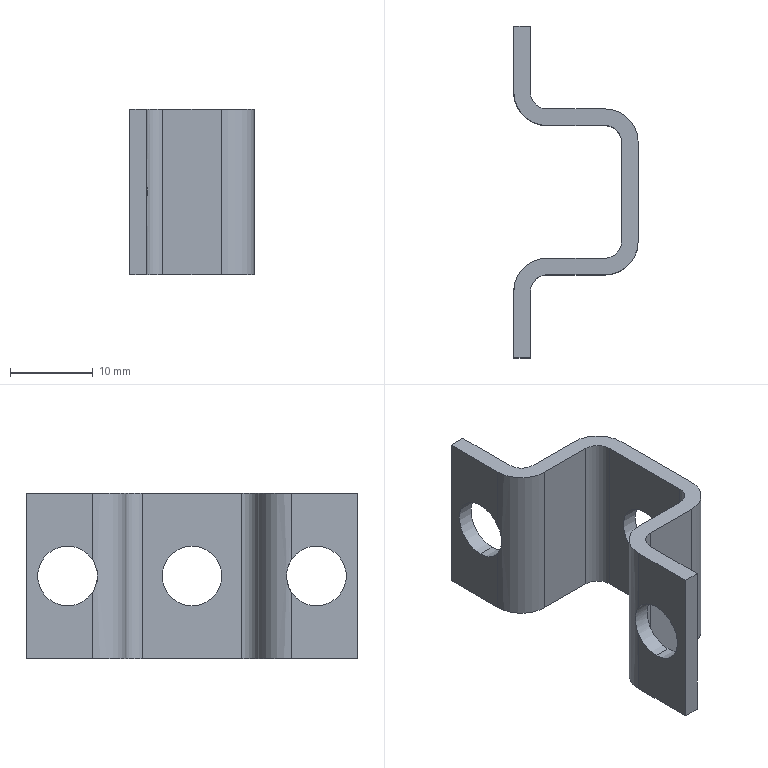Part | NX | features solid 2 | 1 solid | 28 faces | box 15 x 40 x 20 mm | volume 2190 mm3 | cylinder 14 | plane 14 | commonest cylinder face diameters 7.2 x6 4 x4 8 x4
STEP:
#1=CARTESIAN_POINT('',(-1106.,275.,348.4));
#2=VERTEX_POINT('',#1);
#3=CARTESIAN_POINT('',(-1108.,275.,348.4));
#4=VERTEX_POINT('',#3);
#5=CARTESIAN_POINT('',(-1140.17,275.,348.4));
#6=DIRECTION('',(1.,0.,0.));
#7=VECTOR('',#6,1000.);
#8=LINE('',#5,#7);
#9=EDGE_CURVE('',#2,#4,#8,.F.);
#10=ORIENTED_EDGE('',*,*,#9,.T.);
#11=CARTESIAN_POINT('',(-1108.,275.,355.6));
#12=VERTEX_POINT('',#11);
#13=CARTESIAN_POINT('',(-1108.,275.,352.));
#14=DIRECTION('',(-1.,0.,0.));
#15=DIRECTION('',(0.,-1.,0.));
#16=AXIS2_PLACEMENT_3D('',#13,#14,#15);
#17=CIRCLE('',#16,3.6);
#18=EDGE_CURVE('',#4,#12,#17,.T.);
#19=ORIENTED_EDGE('',*,*,#18,.T.);
#20=CARTESIAN_POINT('',(-1106.,275.,355.6));
#21=VERTEX_POINT('',#20);
#22=CARTESIAN_POINT('',(-1140.17,275.,355.6));
#23=DIRECTION('',(1.,0.,0.));
#24=VECTOR('',#23,1000.);
#25=LINE('',#22,#24);
#26=EDGE_CURVE('',#12,#21,#25,.T.);
#27=ORIENTED_EDGE('',*,*,#26,.T.);
#28=CARTESIAN_POINT('',(-1106.,275.,352.));
#29=DIRECTION('',(-1.,0.,0.));
#30=DIRECTION('',(0.,-1.,0.));
#31=AXIS2_PLACEMENT_3D('',#28,#29,#30);
#32=CIRCLE('',#31,3.6);
#33=EDGE_CURVE('',#2,#21,#32,.T.);
#34=ORIENTED_EDGE('',*,*,#33,.F.);
#35=EDGE_LOOP('',(#10,#19,#27,#34));
#36=FACE_BOUND('',#35,.T.);
#37=CARTESIAN_POINT('',(-1140.17,275.,352.));
#38=DIRECTION('',(1.,0.,0.));
#39=DIRECTION('',(0.,0.,1.));
#40=AXIS2_PLACEMENT_3D('',#37,#38,#39);
#41=CYLINDRICAL_SURFACE('',#40,3.6);
#42=ADVANCED_FACE('',(#36),#41,.F.);
#43=CARTESIAN_POINT('',(-1108.,305.,348.4));
#44=VERTEX_POINT('',#43);
#45=CARTESIAN_POINT('',(-1106.,305.,348.4));
#46=VERTEX_POINT('',#45);
#47=CARTESIAN_POINT('',(-1140.17,305.,348.4));
#48=DIRECTION('',(1.,0.,0.));
#49=VECTOR('',#48,1000.);
#50=LINE('',#47,#49);
#51=EDGE_CURVE('',#44,#46,#50,.T.);
#52=ORIENTED_EDGE('',*,*,#51,.F.);
#53=CARTESIAN_POINT('',(-1108.,302.,350.01));
#54=VERTEX_POINT('',#53);
#55=CARTESIAN_POINT('',(-1108.,305.,352.));
#56=DIRECTION('',(-1.,0.,0.));
#57=DIRECTION('',(0.,-1.,0.));
#58=AXIS2_PLACEMENT_3D('',#55,#56,#57);
#59=CIRCLE('',#58,3.6);
#60=EDGE_CURVE('',#44,#54,#59,.T.);
#61=ORIENTED_EDGE('',*,*,#60,.T.);
#62=CARTESIAN_POINT('',(-1108.,302.,353.99));
#63=VERTEX_POINT('',#62);
#64=CARTESIAN_POINT('',(-1108.,302.,350.01));
#65=CARTESIAN_POINT('',(-1108.,301.934,350.109));
#66=CARTESIAN_POINT('',(-1107.997,301.783,350.353));
#67=CARTESIAN_POINT('',(-1107.977,301.531,350.955));
#68=CARTESIAN_POINT('',(-1107.958,301.408,351.604));
#69=CARTESIAN_POINT('',(-1107.953,301.396,351.997));
#70=CARTESIAN_POINT('',(-1107.958,301.408,352.39));
#71=CARTESIAN_POINT('',(-1107.977,301.53,353.043));
#72=CARTESIAN_POINT('',(-1107.997,301.783,353.647));
#73=CARTESIAN_POINT('',(-1108.,301.935,353.891));
#74=CARTESIAN_POINT('',(-1108.,302.,353.99));
#75=B_SPLINE_CURVE_WITH_KNOTS('',3,(#64,#65,#66,#67,#68,#69,#70,#71,#72,#73,#74),.UNSPECIFIED.,.F.,.F.,(4,1,1,1,1,1,1,1,4),(0.,0.125,0.25,0.375,0.5,0.625,0.75,0.875,1.),.UNSPECIFIED.);
#76=EDGE_CURVE('',#54,#63,#75,.T.);
#77=ORIENTED_EDGE('',*,*,#76,.T.);
#78=CARTESIAN_POINT('',(-1108.,305.,355.6));
#79=VERTEX_POINT('',#78);
#80=CARTESIAN_POINT('',(-1108.,305.,352.));
#81=DIRECTION('',(-1.,0.,0.));
#82=DIRECTION('',(0.,-1.,0.));
#83=AXIS2_PLACEMENT_3D('',#80,#81,#82);
#84=CIRCLE('',#83,3.6);
#85=EDGE_CURVE('',#63,#79,#84,.T.);
#86=ORIENTED_EDGE('',*,*,#85,.T.);
#87=CARTESIAN_POINT('',(-1106.,305.,355.6));
#88=VERTEX_POINT('',#87);
#89=CARTESIAN_POINT('',(-1140.17,305.,355.6));
#90=DIRECTION('',(1.,0.,0.));
#91=VECTOR('',#90,1000.);
#92=LINE('',#89,#91);
#93=EDGE_CURVE('',#88,#79,#92,.F.);
#94=ORIENTED_EDGE('',*,*,#93,.F.);
#95=CARTESIAN_POINT('',(-1106.,302.,353.99));
#96=VERTEX_POINT('',#95);
#97=CARTESIAN_POINT('',(-1106.,305.,352.));
#98=DIRECTION('',(-1.,0.,0.));
#99=DIRECTION('',(0.,-1.,0.));
#100=AXIS2_PLACEMENT_3D('',#97,#98,#99);
#101=CIRCLE('',#100,3.6);
#102=EDGE_CURVE('',#96,#88,#101,.T.);
#103=ORIENTED_EDGE('',*,*,#102,.F.);
#104=CARTESIAN_POINT('',(-1106.,302.,350.01));
#105=VERTEX_POINT('',#104);
#106=CARTESIAN_POINT('',(-1106.,302.,353.99));
#107=CARTESIAN_POINT('',(-1106.,301.948,353.912));
#108=CARTESIAN_POINT('',(-1105.993,301.807,353.704));
#109=CARTESIAN_POINT('',(-1105.929,301.427,352.772));
#110=CARTESIAN_POINT('',(-1105.894,301.382,351.998));
#111=CARTESIAN_POINT('',(-1105.929,301.428,351.227));
#112=CARTESIAN_POINT('',(-1105.993,301.808,350.296));
#113=CARTESIAN_POINT('',(-1106.,301.948,350.088));
#114=CARTESIAN_POINT('',(-1106.,302.,350.01));
#115=B_SPLINE_CURVE_WITH_KNOTS('',3,(#106,#107,#108,#109,#110,#111,#112,#113,#114),.UNSPECIFIED.,.F.,.F.,(4,1,1,1,1,1,4),(0.,0.125,0.25,0.5,0.75,0.875,1.),.UNSPECIFIED.);
#116=EDGE_CURVE('',#105,#96,#115,.F.);
#117=ORIENTED_EDGE('',*,*,#116,.F.);
#118=CARTESIAN_POINT('',(-1106.,305.,352.));
#119=DIRECTION('',(-1.,0.,0.));
#120=DIRECTION('',(0.,-1.,0.));
#121=AXIS2_PLACEMENT_3D('',#118,#119,#120);
#122=CIRCLE('',#121,3.6);
#123=EDGE_CURVE('',#46,#105,#122,.T.);
#124=ORIENTED_EDGE('',*,*,#123,.F.);
#125=EDGE_LOOP('',(#52,#61,#77,#86,#94,#103,#117,#124));
#126=FACE_BOUND('',#125,.T.);
#127=CARTESIAN_POINT('',(-1140.17,305.,352.));
#128=DIRECTION('',(1.,0.,0.));
#129=DIRECTION('',(0.,0.,1.));
#130=AXIS2_PLACEMENT_3D('',#127,#128,#129);
#131=CYLINDRICAL_SURFACE('',#130,3.6);
#132=ADVANCED_FACE('',(#126),#131,.F.);
#133=CARTESIAN_POINT('',(-1095.,290.,348.4));
#134=VERTEX_POINT('',#133);
#135=CARTESIAN_POINT('',(-1093.,290.,348.4));
#136=VERTEX_POINT('',#135);
#137=CARTESIAN_POINT('',(-1140.17,290.,348.4));
#138=DIRECTION('',(1.,0.,0.));
#139=VECTOR('',#138,1000.);
#140=LINE('',#137,#139);
#141=EDGE_CURVE('',#134,#136,#140,.T.);
#142=ORIENTED_EDGE('',*,*,#141,.F.);
#143=CARTESIAN_POINT('',(-1095.,290.,355.6));
#144=VERTEX_POINT('',#143);
#145=CARTESIAN_POINT('',(-1095.,290.,352.));
#146=DIRECTION('',(-1.,0.,0.));
#147=DIRECTION('',(0.,0.,-1.));
#148=AXIS2_PLACEMENT_3D('',#145,#146,#147);
#149=CIRCLE('',#148,3.6);
#150=EDGE_CURVE('',#134,#144,#149,.T.);
#151=ORIENTED_EDGE('',*,*,#150,.T.);
#152=CARTESIAN_POINT('',(-1093.,290.,355.6));
#153=VERTEX_POINT('',#152);
#154=CARTESIAN_POINT('',(-1140.17,290.,355.6));
#155=DIRECTION('',(1.,0.,0.));
#156=VECTOR('',#155,1000.);
#157=LINE('',#154,#156);
#158=EDGE_CURVE('',#153,#144,#157,.F.);
#159=ORIENTED_EDGE('',*,*,#158,.F.);
#160=CARTESIAN_POINT('',(-1093.,290.,352.));
#161=DIRECTION('',(1.,0.,0.));
#162=DIRECTION('',(0.,-1.,0.));
#163=AXIS2_PLACEMENT_3D('',#160,#161,#162);
#164=CIRCLE('',#163,3.6);
#165=EDGE_CURVE('',#153,#136,#164,.T.);
#166=ORIENTED_EDGE('',*,*,#165,.T.);
#167=EDGE_LOOP('',(#142,#151,#159,#166));
#168=FACE_BOUND('',#167,.T.);
#169=CARTESIAN_POINT('',(-1140.17,290.,352.));
#170=DIRECTION('',(1.,0.,0.));
#171=DIRECTION('',(0.,0.,1.));
#172=AXIS2_PLACEMENT_3D('',#169,#170,#171);
#173=CYLINDRICAL_SURFACE('',#172,3.6);
#174=ADVANCED_FACE('',(#168),#173,.F.);
#175=CARTESIAN_POINT('',(-1106.,302.,342.));
#176=VERTEX_POINT('',#175);
#177=CARTESIAN_POINT('',(-1106.,302.,342.));
#178=DIRECTION('',(0.,0.,1.));
#179=VECTOR('',#178,1000.);
#180=LINE('',#177,#179);
#181=EDGE_CURVE('',#176,#105,#180,.T.);
#182=ORIENTED_EDGE('',*,*,#181,.T.);
#183=ORIENTED_EDGE('',*,*,#116,.T.);
#184=CARTESIAN_POINT('',(-1106.,302.,362.));
#185=VERTEX_POINT('',#184);
#186=CARTESIAN_POINT('',(-1106.,302.,342.));
#187=DIRECTION('',(0.,0.,1.));
#188=VECTOR('',#187,1000.);
#189=LINE('',#186,#188);
#190=EDGE_CURVE('',#96,#185,#189,.T.);
#191=ORIENTED_EDGE('',*,*,#190,.T.);
#192=CARTESIAN_POINT('',(-1104.,300.,362.));
#193=VERTEX_POINT('',#192);
#194=CARTESIAN_POINT('',(-1104.,302.,362.));
#195=DIRECTION('',(0.,0.,1.));
#196=DIRECTION('',(1.,0.,0.));
#197=AXIS2_PLACEMENT_3D('',#194,#195,#196);
#198=CIRCLE('',#197,2.);
#199=EDGE_CURVE('',#185,#193,#198,.T.);
#200=ORIENTED_EDGE('',*,*,#199,.T.);
#201=CARTESIAN_POINT('',(-1104.,300.,342.));
#202=VERTEX_POINT('',#201);
#203=CARTESIAN_POINT('',(-1104.,300.,362.));
#204=DIRECTION('',(0.,0.,-1.));
#205=VECTOR('',#204,1000.);
#206=LINE('',#203,#205);
#207=EDGE_CURVE('',#193,#202,#206,.T.);
#208=ORIENTED_EDGE('',*,*,#207,.T.);
#209=CARTESIAN_POINT('',(-1104.,302.,342.));
#210=DIRECTION('',(0.,0.,1.));
#211=DIRECTION('',(1.,0.,0.));
#212=AXIS2_PLACEMENT_3D('',#209,#210,#211);
#213=CIRCLE('',#212,2.);
#214=EDGE_CURVE('',#176,#202,#213,.T.);
#215=ORIENTED_EDGE('',*,*,#214,.F.);
#216=EDGE_LOOP('',(#182,#183,#191,#200,#208,#215));
#217=FACE_BOUND('',#216,.T.);
#218=CARTESIAN_POINT('',(-1104.,302.,362.));
#219=DIRECTION('',(0.,0.,-1.));
#220=DIRECTION('',(0.,1.,0.));
#221=AXIS2_PLACEMENT_3D('',#218,#219,#220);
#222=CYLINDRICAL_SURFACE('',#221,2.);
#223=ADVANCED_FACE('',(#217),#222,.F.);
#224=ORIENTED_EDGE('',*,*,#76,.F.);
#225=CARTESIAN_POINT('',(-1108.,302.,342.));
#226=VERTEX_POINT('',#225);
#227=CARTESIAN_POINT('',(-1108.,302.,342.));
#228=DIRECTION('',(0.,0.,1.));
#229=VECTOR('',#228,1000.);
#230=LINE('',#227,#229);
#231=EDGE_CURVE('',#226,#54,#230,.T.);
#232=ORIENTED_EDGE('',*,*,#231,.F.);
#233=CARTESIAN_POINT('',(-1104.,298.,342.));
#234=VERTEX_POINT('',#233);
#235=CARTESIAN_POINT('',(-1104.,302.,342.));
#236=DIRECTION('',(0.,0.,1.));
#237=DIRECTION('',(0.,1.,0.));
#238=AXIS2_PLACEMENT_3D('',#235,#236,#237);
#239=CIRCLE('',#238,4.);
#240=EDGE_CURVE('',#226,#234,#239,.T.);
#241=ORIENTED_EDGE('',*,*,#240,.T.);
#242=CARTESIAN_POINT('',(-1104.,298.,362.));
#243=VERTEX_POINT('',#242);
#244=CARTESIAN_POINT('',(-1104.,298.,362.));
#245=DIRECTION('',(0.,0.,-1.));
#246=VECTOR('',#245,1000.);
#247=LINE('',#244,#246);
#248=EDGE_CURVE('',#243,#234,#247,.T.);
#249=ORIENTED_EDGE('',*,*,#248,.F.);
#250=CARTESIAN_POINT('',(-1108.,302.,362.));
#251=VERTEX_POINT('',#250);
#252=CARTESIAN_POINT('',(-1104.,302.,362.));
#253=DIRECTION('',(0.,0.,1.));
#254=DIRECTION('',(0.,1.,0.));
#255=AXIS2_PLACEMENT_3D('',#252,#253,#254);
#256=CIRCLE('',#255,4.);
#257=EDGE_CURVE('',#251,#243,#256,.T.);
#258=ORIENTED_EDGE('',*,*,#257,.F.);
#259=CARTESIAN_POINT('',(-1108.,302.,342.));
#260=DIRECTION('',(0.,0.,1.));
#261=VECTOR('',#260,1000.);
#262=LINE('',#259,#261);
#263=EDGE_CURVE('',#63,#251,#262,.T.);
#264=ORIENTED_EDGE('',*,*,#263,.F.);
#265=EDGE_LOOP('',(#224,#232,#241,#249,#258,#264));
#266=FACE_BOUND('',#265,.T.);
#267=CARTESIAN_POINT('',(-1104.,302.,362.));
#268=DIRECTION('',(0.,0.,-1.));
#269=DIRECTION('',(0.,1.,0.));
#270=AXIS2_PLACEMENT_3D('',#267,#268,#269);
#271=CYLINDRICAL_SURFACE('',#270,4.);
#272=ADVANCED_FACE('',(#266),#271,.T.);
#273=CARTESIAN_POINT('',(-1106.,310.,362.));
#274=VERTEX_POINT('',#273);
#275=CARTESIAN_POINT('',(-1106.,310.,342.));
#276=VERTEX_POINT('',#275);
#277=CARTESIAN_POINT('',(-1106.,310.,362.));
#278=DIRECTION('',(0.,0.,-1.));
#279=VECTOR('',#278,1000.);
#280=LINE('',#277,#279);
#281=EDGE_CURVE('',#274,#276,#280,.T.);
#282=ORIENTED_EDGE('',*,*,#281,.T.);
#283=CARTESIAN_POINT('',(-1108.,310.,342.));
#284=VERTEX_POINT('',#283);
#285=CARTESIAN_POINT('',(-1108.,310.,342.));
#286=DIRECTION('',(1.,0.,0.));
#287=VECTOR('',#286,1000.);
#288=LINE('',#285,#287);
#289=EDGE_CURVE('',#284,#276,#288,.T.);
#290=ORIENTED_EDGE('',*,*,#289,.F.);
#291=CARTESIAN_POINT('',(-1108.,310.,362.));
#292=VERTEX_POINT('',#291);
#293=CARTESIAN_POINT('',(-1108.,310.,362.));
#294=DIRECTION('',(0.,0.,-1.));
#295=VECTOR('',#294,1000.);
#296=LINE('',#293,#295);
#297=EDGE_CURVE('',#292,#284,#296,.T.);
#298=ORIENTED_EDGE('',*,*,#297,.F.);
#299=CARTESIAN_POINT('',(-1108.,310.,362.));
#300=DIRECTION('',(1.,0.,0.));
#301=VECTOR('',#300,1000.);
#302=LINE('',#299,#301);
#303=EDGE_CURVE('',#292,#274,#302,.T.);
#304=ORIENTED_EDGE('',*,*,#303,.T.);
#305=EDGE_LOOP('',(#282,#290,#298,#304));
#306=FACE_BOUND('',#305,.T.);
#307=CARTESIAN_POINT('',(-1108.,310.,362.));
#308=DIRECTION('',(0.,-1.,0.));
#309=DIRECTION('',(0.,0.,-1.));
#310=AXIS2_PLACEMENT_3D('',#307,#308,#309);
#311=PLANE('',#310);
#312=ADVANCED_FACE('',(#306),#311,.F.);
#313=ORIENTED_EDGE('',*,*,#190,.F.);
#314=ORIENTED_EDGE('',*,*,#102,.T.);
#315=CARTESIAN_POINT('',(-1106.,305.,352.));
#316=DIRECTION('',(-1.,0.,0.));
#317=DIRECTION('',(0.,-1.,0.));
#318=AXIS2_PLACEMENT_3D('',#315,#316,#317);
#319=CIRCLE('',#318,3.6);
#320=EDGE_CURVE('',#88,#46,#319,.T.);
#321=ORIENTED_EDGE('',*,*,#320,.T.);
#322=ORIENTED_EDGE('',*,*,#123,.T.);
#323=ORIENTED_EDGE('',*,*,#181,.F.);
#324=CARTESIAN_POINT('',(-1106.,299.722,342.));
#325=DIRECTION('',(0.,-1.,0.));
#326=VECTOR('',#325,1000.);
#327=LINE('',#324,#326);
#328=EDGE_CURVE('',#276,#176,#327,.T.);
#329=ORIENTED_EDGE('',*,*,#328,.F.);
#330=ORIENTED_EDGE('',*,*,#281,.F.);
#331=CARTESIAN_POINT('',(-1106.,299.722,362.));
#332=DIRECTION('',(0.,1.,0.));
#333=VECTOR('',#332,1000.);
#334=LINE('',#331,#333);
#335=EDGE_CURVE('',#185,#274,#334,.T.);
#336=ORIENTED_EDGE('',*,*,#335,.F.);
#337=EDGE_LOOP('',(#313,#314,#321,#322,#323,#329,#330,#336));
#338=FACE_BOUND('',#337,.T.);
#339=CARTESIAN_POINT('',(-1106.,290.,352.));
#340=DIRECTION('',(-1.,0.,0.));
#341=DIRECTION('',(0.,1.,0.));
#342=AXIS2_PLACEMENT_3D('',#339,#340,#341);
#343=PLANE('',#342);
#344=ADVANCED_FACE('',(#338),#343,.F.);
#345=ORIENTED_EDGE('',*,*,#85,.F.);
#346=ORIENTED_EDGE('',*,*,#263,.T.);
#347=CARTESIAN_POINT('',(-1108.,299.722,362.));
#348=DIRECTION('',(0.,1.,0.));
#349=VECTOR('',#348,1000.);
#350=LINE('',#347,#349);
#351=EDGE_CURVE('',#251,#292,#350,.T.);
#352=ORIENTED_EDGE('',*,*,#351,.T.);
#353=ORIENTED_EDGE('',*,*,#297,.T.);
#354=CARTESIAN_POINT('',(-1108.,299.722,342.));
#355=DIRECTION('',(0.,-1.,0.));
#356=VECTOR('',#355,1000.);
#357=LINE('',#354,#356);
#358=EDGE_CURVE('',#284,#226,#357,.T.);
#359=ORIENTED_EDGE('',*,*,#358,.T.);
#360=ORIENTED_EDGE('',*,*,#231,.T.);
#361=ORIENTED_EDGE('',*,*,#60,.F.);
#362=CARTESIAN_POINT('',(-1108.,305.,352.));
#363=DIRECTION('',(-1.,0.,0.));
#364=DIRECTION('',(0.,-1.,0.));
#365=AXIS2_PLACEMENT_3D('',#362,#363,#364);
#366=CIRCLE('',#365,3.6);
#367=EDGE_CURVE('',#79,#44,#366,.T.);
#368=ORIENTED_EDGE('',*,*,#367,.F.);
#369=EDGE_LOOP('',(#345,#346,#352,#353,#359,#360,#361,#368));
#370=FACE_BOUND('',#369,.T.);
#371=CARTESIAN_POINT('',(-1108.,290.,352.));
#372=DIRECTION('',(-1.,0.,0.));
#373=DIRECTION('',(0.,1.,0.));
#374=AXIS2_PLACEMENT_3D('',#371,#372,#373);
#375=PLANE('',#374);
#376=ADVANCED_FACE('',(#370),#375,.T.);
#377=CARTESIAN_POINT('',(-1106.,278.,362.));
#378=VERTEX_POINT('',#377);
#379=CARTESIAN_POINT('',(-1106.,278.,353.99));
#380=VERTEX_POINT('',#379);
#381=CARTESIAN_POINT('',(-1106.,278.,362.));
#382=DIRECTION('',(0.,0.,-1.));
#383=VECTOR('',#382,1000.);
#384=LINE('',#381,#383);
#385=EDGE_CURVE('',#378,#380,#384,.T.);
#386=ORIENTED_EDGE('',*,*,#385,.T.);
#387=CARTESIAN_POINT('',(-1106.,278.,350.01));
#388=VERTEX_POINT('',#387);
#389=CARTESIAN_POINT('',(-1106.,278.,353.99));
#390=CARTESIAN_POINT('',(-1106.,278.406,353.378));
#391=CARTESIAN_POINT('',(-1105.816,278.794,352.002));
#392=CARTESIAN_POINT('',(-1106.,278.406,350.623));
#393=CARTESIAN_POINT('',(-1106.,278.,350.01));
#394=B_SPLINE_CURVE_WITH_KNOTS('',3,(#389,#390,#391,#392,#393),.UNSPECIFIED.,.F.,.F.,(4,1,4),(0.,0.5,1.),.UNSPECIFIED.);
#395=EDGE_CURVE('',#380,#388,#394,.T.);
#396=ORIENTED_EDGE('',*,*,#395,.T.);
#397=CARTESIAN_POINT('',(-1106.,278.,342.));
#398=VERTEX_POINT('',#397);
#399=CARTESIAN_POINT('',(-1106.,278.,362.));
#400=DIRECTION('',(0.,0.,-1.));
#401=VECTOR('',#400,1000.);
#402=LINE('',#399,#401);
#403=EDGE_CURVE('',#388,#398,#402,.T.);
#404=ORIENTED_EDGE('',*,*,#403,.T.);
#405=CARTESIAN_POINT('',(-1104.,280.,342.));
#406=VERTEX_POINT('',#405);
#407=CARTESIAN_POINT('',(-1104.,278.,342.));
#408=DIRECTION('',(0.,0.,1.));
#409=DIRECTION('',(-1.,0.,0.));
#410=AXIS2_PLACEMENT_3D('',#407,#408,#409);
#411=CIRCLE('',#410,2.);
#412=EDGE_CURVE('',#406,#398,#411,.T.);
#413=ORIENTED_EDGE('',*,*,#412,.F.);
#414=CARTESIAN_POINT('',(-1104.,280.,362.));
#415=VERTEX_POINT('',#414);
#416=CARTESIAN_POINT('',(-1104.,280.,342.));
#417=DIRECTION('',(0.,0.,1.));
#418=VECTOR('',#417,1000.);
#419=LINE('',#416,#418);
#420=EDGE_CURVE('',#406,#415,#419,.T.);
#421=ORIENTED_EDGE('',*,*,#420,.T.);
#422=CARTESIAN_POINT('',(-1104.,278.,362.));
#423=DIRECTION('',(0.,0.,1.));
#424=DIRECTION('',(-1.,0.,0.));
#425=AXIS2_PLACEMENT_3D('',#422,#423,#424);
#426=CIRCLE('',#425,2.);
#427=EDGE_CURVE('',#415,#378,#426,.T.);
#428=ORIENTED_EDGE('',*,*,#427,.T.);
#429=EDGE_LOOP('',(#386,#396,#404,#413,#421,#428));
#430=FACE_BOUND('',#429,.T.);
#431=CARTESIAN_POINT('',(-1104.,278.,342.));
#432=DIRECTION('',(0.,0.,1.));
#433=DIRECTION('',(0.,-1.,0.));
#434=AXIS2_PLACEMENT_3D('',#431,#432,#433);
#435=CYLINDRICAL_SURFACE('',#434,2.);
#436=ADVANCED_FACE('',(#430),#435,.F.);
#437=CARTESIAN_POINT('',(-1108.,278.,353.99));
#438=VERTEX_POINT('',#437);
#439=CARTESIAN_POINT('',(-1108.,278.,350.01));
#440=VERTEX_POINT('',#439);
#441=CARTESIAN_POINT('',(-1108.,278.,350.01));
#442=CARTESIAN_POINT('',(-1108.,278.402,350.616));
#443=CARTESIAN_POINT('',(-1107.909,278.798,352.006));
#444=CARTESIAN_POINT('',(-1108.,278.401,353.385));
#445=CARTESIAN_POINT('',(-1108.,278.,353.99));
#446=B_SPLINE_CURVE_WITH_KNOTS('',3,(#441,#442,#443,#444,#445),.UNSPECIFIED.,.F.,.F.,(4,1,4),(0.,0.5,1.),.UNSPECIFIED.);
#447=EDGE_CURVE('',#438,#440,#446,.F.);
#448=ORIENTED_EDGE('',*,*,#447,.F.);
#449=CARTESIAN_POINT('',(-1108.,278.,362.));
#450=VERTEX_POINT('',#449);
#451=CARTESIAN_POINT('',(-1108.,278.,362.));
#452=DIRECTION('',(0.,0.,-1.));
#453=VECTOR('',#452,1000.);
#454=LINE('',#451,#453);
#455=EDGE_CURVE('',#450,#438,#454,.T.);
#456=ORIENTED_EDGE('',*,*,#455,.F.);
#457=CARTESIAN_POINT('',(-1104.,282.,362.));
#458=VERTEX_POINT('',#457);
#459=CARTESIAN_POINT('',(-1104.,278.,362.));
#460=DIRECTION('',(0.,0.,1.));
#461=DIRECTION('',(0.,-1.,0.));
#462=AXIS2_PLACEMENT_3D('',#459,#460,#461);
#463=CIRCLE('',#462,4.);
#464=EDGE_CURVE('',#458,#450,#463,.T.);
#465=ORIENTED_EDGE('',*,*,#464,.F.);
#466=CARTESIAN_POINT('',(-1104.,282.,342.));
#467=VERTEX_POINT('',#466);
#468=CARTESIAN_POINT('',(-1104.,282.,342.));
#469=DIRECTION('',(0.,0.,1.));
#470=VECTOR('',#469,1000.);
#471=LINE('',#468,#470);
#472=EDGE_CURVE('',#467,#458,#471,.T.);
#473=ORIENTED_EDGE('',*,*,#472,.F.);
#474=CARTESIAN_POINT('',(-1108.,278.,342.));
#475=VERTEX_POINT('',#474);
#476=CARTESIAN_POINT('',(-1104.,278.,342.));
#477=DIRECTION('',(0.,0.,1.));
#478=DIRECTION('',(0.,-1.,0.));
#479=AXIS2_PLACEMENT_3D('',#476,#477,#478);
#480=CIRCLE('',#479,4.);
#481=EDGE_CURVE('',#467,#475,#480,.T.);
#482=ORIENTED_EDGE('',*,*,#481,.T.);
#483=CARTESIAN_POINT('',(-1108.,278.,362.));
#484=DIRECTION('',(0.,0.,-1.));
#485=VECTOR('',#484,1000.);
#486=LINE('',#483,#485);
#487=EDGE_CURVE('',#440,#475,#486,.T.);
#488=ORIENTED_EDGE('',*,*,#487,.F.);
#489=EDGE_LOOP('',(#448,#456,#465,#473,#482,#488));
#490=FACE_BOUND('',#489,.T.);
#491=CARTESIAN_POINT('',(-1104.,278.,342.));
#492=DIRECTION('',(0.,0.,1.));
#493=DIRECTION('',(0.,-1.,0.));
#494=AXIS2_PLACEMENT_3D('',#491,#492,#493);
#495=CYLINDRICAL_SURFACE('',#494,4.);
#496=ADVANCED_FACE('',(#490),#495,.T.);
#497=CARTESIAN_POINT('',(-1106.,270.,342.));
#498=VERTEX_POINT('',#497);
#499=CARTESIAN_POINT('',(-1106.,270.,362.));
#500=VERTEX_POINT('',#499);
#501=CARTESIAN_POINT('',(-1106.,270.,342.));
#502=DIRECTION('',(0.,0.,1.));
#503=VECTOR('',#502,1000.);
#504=LINE('',#501,#503);
#505=EDGE_CURVE('',#498,#500,#504,.T.);
#506=ORIENTED_EDGE('',*,*,#505,.T.);
#507=CARTESIAN_POINT('',(-1108.,270.,362.));
#508=VERTEX_POINT('',#507);
#509=CARTESIAN_POINT('',(-1108.,270.,362.));
#510=DIRECTION('',(1.,0.,0.));
#511=VECTOR('',#510,1000.);
#512=LINE('',#509,#511);
#513=EDGE_CURVE('',#508,#500,#512,.T.);
#514=ORIENTED_EDGE('',*,*,#513,.F.);
#515=CARTESIAN_POINT('',(-1108.,270.,342.));
#516=VERTEX_POINT('',#515);
#517=CARTESIAN_POINT('',(-1108.,270.,342.));
#518=DIRECTION('',(0.,0.,1.));
#519=VECTOR('',#518,1000.);
#520=LINE('',#517,#519);
#521=EDGE_CURVE('',#516,#508,#520,.T.);
#522=ORIENTED_EDGE('',*,*,#521,.F.);
#523=CARTESIAN_POINT('',(-1108.,270.,342.));
#524=DIRECTION('',(1.,0.,0.));
#525=VECTOR('',#524,1000.);
#526=LINE('',#523,#525);
#527=EDGE_CURVE('',#516,#498,#526,.T.);
#528=ORIENTED_EDGE('',*,*,#527,.T.);
#529=EDGE_LOOP('',(#506,#514,#522,#528));
#530=FACE_BOUND('',#529,.T.);
#531=CARTESIAN_POINT('',(-1108.,270.,342.));
#532=DIRECTION('',(0.,1.,0.));
#533=DIRECTION('',(1.,0.,0.));
#534=AXIS2_PLACEMENT_3D('',#531,#532,#533);
#535=PLANE('',#534);
#536=ADVANCED_FACE('',(#530),#535,.F.);
#537=ORIENTED_EDGE('',*,*,#403,.F.);
#538=CARTESIAN_POINT('',(-1106.,275.,352.));
#539=DIRECTION('',(-1.,0.,0.));
#540=DIRECTION('',(0.,-1.,0.));
#541=AXIS2_PLACEMENT_3D('',#538,#539,#540);
#542=CIRCLE('',#541,3.6);
#543=EDGE_CURVE('',#388,#2,#542,.T.);
#544=ORIENTED_EDGE('',*,*,#543,.T.);
#545=ORIENTED_EDGE('',*,*,#33,.T.);
#546=CARTESIAN_POINT('',(-1106.,275.,352.));
#547=DIRECTION('',(-1.,0.,0.));
#548=DIRECTION('',(0.,-1.,0.));
#549=AXIS2_PLACEMENT_3D('',#546,#547,#548);
#550=CIRCLE('',#549,3.6);
#551=EDGE_CURVE('',#21,#380,#550,.T.);
#552=ORIENTED_EDGE('',*,*,#551,.T.);
#553=ORIENTED_EDGE('',*,*,#385,.F.);
#554=CARTESIAN_POINT('',(-1106.,280.278,362.));
#555=DIRECTION('',(0.,1.,0.));
#556=VECTOR('',#555,1000.);
#557=LINE('',#554,#556);
#558=EDGE_CURVE('',#500,#378,#557,.T.);
#559=ORIENTED_EDGE('',*,*,#558,.F.);
#560=ORIENTED_EDGE('',*,*,#505,.F.);
#561=CARTESIAN_POINT('',(-1106.,280.278,342.));
#562=DIRECTION('',(0.,-1.,0.));
#563=VECTOR('',#562,1000.);
#564=LINE('',#561,#563);
#565=EDGE_CURVE('',#398,#498,#564,.T.);
#566=ORIENTED_EDGE('',*,*,#565,.F.);
#567=EDGE_LOOP('',(#537,#544,#545,#552,#553,#559,#560,#566));
#568=FACE_BOUND('',#567,.T.);
#569=CARTESIAN_POINT('',(-1106.,290.,352.));
#570=DIRECTION('',(-1.,0.,0.));
#571=DIRECTION('',(0.,0.,1.));
#572=AXIS2_PLACEMENT_3D('',#569,#570,#571);
#573=PLANE('',#572);
#574=ADVANCED_FACE('',(#568),#573,.F.);
#575=CARTESIAN_POINT('',(-1108.,275.,352.));
#576=DIRECTION('',(-1.,0.,0.));
#577=DIRECTION('',(0.,-1.,0.));
#578=AXIS2_PLACEMENT_3D('',#575,#576,#577);
#579=CIRCLE('',#578,3.6);
#580=EDGE_CURVE('',#440,#4,#579,.T.);
#581=ORIENTED_EDGE('',*,*,#580,.F.);
#582=ORIENTED_EDGE('',*,*,#487,.T.);
#583=CARTESIAN_POINT('',(-1108.,280.278,342.));
#584=DIRECTION('',(0.,-1.,0.));
#585=VECTOR('',#584,1000.);
#586=LINE('',#583,#585);
#587=EDGE_CURVE('',#475,#516,#586,.T.);
#588=ORIENTED_EDGE('',*,*,#587,.T.);
#589=ORIENTED_EDGE('',*,*,#521,.T.);
#590=CARTESIAN_POINT('',(-1108.,280.278,362.));
#591=DIRECTION('',(0.,1.,0.));
#592=VECTOR('',#591,1000.);
#593=LINE('',#590,#592);
#594=EDGE_CURVE('',#508,#450,#593,.T.);
#595=ORIENTED_EDGE('',*,*,#594,.T.);
#596=ORIENTED_EDGE('',*,*,#455,.T.);
#597=CARTESIAN_POINT('',(-1108.,275.,352.));
#598=DIRECTION('',(-1.,0.,0.));
#599=DIRECTION('',(0.,-1.,0.));
#600=AXIS2_PLACEMENT_3D('',#597,#598,#599);
#601=CIRCLE('',#600,3.6);
#602=EDGE_CURVE('',#12,#438,#601,.T.);
#603=ORIENTED_EDGE('',*,*,#602,.F.);
#604=ORIENTED_EDGE('',*,*,#18,.F.);
#605=EDGE_LOOP('',(#581,#582,#588,#589,#595,#596,#603,#604));
#606=FACE_BOUND('',#605,.T.);
#607=CARTESIAN_POINT('',(-1108.,290.,352.));
#608=DIRECTION('',(-1.,0.,0.));
#609=DIRECTION('',(0.,0.,1.));
#610=AXIS2_PLACEMENT_3D('',#607,#608,#609);
#611=PLANE('',#610);
#612=ADVANCED_FACE('',(#606),#611,.T.);
#613=ORIENTED_EDGE('',*,*,#420,.F.);
#614=CARTESIAN_POINT('',(-1097.,280.,342.));
#615=VERTEX_POINT('',#614);
#616=CARTESIAN_POINT('',(-1108.,280.,342.));
#617=DIRECTION('',(-1.,0.,0.));
#618=VECTOR('',#617,1000.);
#619=LINE('',#616,#618);
#620=EDGE_CURVE('',#615,#406,#619,.T.);
#621=ORIENTED_EDGE('',*,*,#620,.F.);
#622=CARTESIAN_POINT('',(-1097.,280.,362.));
#623=VERTEX_POINT('',#622);
#624=CARTESIAN_POINT('',(-1097.,280.,342.));
#625=DIRECTION('',(0.,0.,1.));
#626=VECTOR('',#625,1000.);
#627=LINE('',#624,#626);
#628=EDGE_CURVE('',#615,#623,#627,.T.);
#629=ORIENTED_EDGE('',*,*,#628,.T.);
#630=CARTESIAN_POINT('',(-1108.,280.,362.));
#631=DIRECTION('',(-1.,0.,0.));
#632=VECTOR('',#631,1000.);
#633=LINE('',#630,#632);
#634=EDGE_CURVE('',#623,#415,#633,.T.);
#635=ORIENTED_EDGE('',*,*,#634,.T.);
#636=EDGE_LOOP('',(#613,#621,#629,#635));
#637=FACE_BOUND('',#636,.T.);
#638=CARTESIAN_POINT('',(-1108.,280.,342.));
#639=DIRECTION('',(0.,1.,0.));
#640=DIRECTION('',(1.,0.,0.));
#641=AXIS2_PLACEMENT_3D('',#638,#639,#640);
#642=PLANE('',#641);
#643=ADVANCED_FACE('',(#637),#642,.F.);
#644=CARTESIAN_POINT('',(-1093.,284.,362.));
#645=VERTEX_POINT('',#644);
#646=CARTESIAN_POINT('',(-1097.,284.,362.));
#647=DIRECTION('',(0.,0.,-1.));
#648=DIRECTION('',(-1.,0.,0.));
#649=AXIS2_PLACEMENT_3D('',#646,#647,#648);
#650=CIRCLE('',#649,4.);
#651=EDGE_CURVE('',#645,#623,#650,.T.);
#652=ORIENTED_EDGE('',*,*,#651,.T.);
#653=ORIENTED_EDGE('',*,*,#628,.F.);
#654=CARTESIAN_POINT('',(-1093.,284.,342.));
#655=VERTEX_POINT('',#654);
#656=CARTESIAN_POINT('',(-1097.,284.,342.));
#657=DIRECTION('',(0.,0.,-1.));
#658=DIRECTION('',(-1.,0.,0.));
#659=AXIS2_PLACEMENT_3D('',#656,#657,#658);
#660=CIRCLE('',#659,4.);
#661=EDGE_CURVE('',#655,#615,#660,.T.);
#662=ORIENTED_EDGE('',*,*,#661,.F.);
#663=CARTESIAN_POINT('',(-1093.,284.,342.));
#664=DIRECTION('',(0.,0.,1.));
#665=VECTOR('',#664,1000.);
#666=LINE('',#663,#665);
#667=EDGE_CURVE('',#655,#645,#666,.T.);
#668=ORIENTED_EDGE('',*,*,#667,.T.);
#669=EDGE_LOOP('',(#652,#653,#662,#668));
#670=FACE_BOUND('',#669,.T.);
#671=CARTESIAN_POINT('',(-1097.,284.,342.));
#672=DIRECTION('',(0.,0.,1.));
#673=DIRECTION('',(-1.,0.,0.));
#674=AXIS2_PLACEMENT_3D('',#671,#672,#673);
#675=CYLINDRICAL_SURFACE('',#674,4.);
#676=ADVANCED_FACE('',(#670),#675,.T.);
#677=ORIENTED_EDGE('',*,*,#165,.F.);
#678=CARTESIAN_POINT('',(-1093.,290.,352.));
#679=DIRECTION('',(1.,0.,0.));
#680=DIRECTION('',(0.,-1.,0.));
#681=AXIS2_PLACEMENT_3D('',#678,#679,#680);
#682=CIRCLE('',#681,3.6);
#683=EDGE_CURVE('',#136,#153,#682,.T.);
#684=ORIENTED_EDGE('',*,*,#683,.F.);
#685=EDGE_LOOP('',(#677,#684));
#686=FACE_BOUND('',#685,.T.);
#687=CARTESIAN_POINT('',(-1093.,296.,362.));
#688=VERTEX_POINT('',#687);
#689=CARTESIAN_POINT('',(-1093.,280.,362.));
#690=DIRECTION('',(0.,-1.,0.));
#691=VECTOR('',#690,1000.);
#692=LINE('',#689,#691);
#693=EDGE_CURVE('',#688,#645,#692,.T.);
#694=ORIENTED_EDGE('',*,*,#693,.T.);
#695=ORIENTED_EDGE('',*,*,#667,.F.);
#696=CARTESIAN_POINT('',(-1093.,296.,342.));
#697=VERTEX_POINT('',#696);
#698=CARTESIAN_POINT('',(-1093.,280.,342.));
#699=DIRECTION('',(0.,-1.,0.));
#700=VECTOR('',#699,1000.);
#701=LINE('',#698,#700);
#702=EDGE_CURVE('',#697,#655,#701,.T.);
#703=ORIENTED_EDGE('',*,*,#702,.F.);
#704=CARTESIAN_POINT('',(-1093.,296.,342.));
#705=DIRECTION('',(0.,0.,1.));
#706=VECTOR('',#705,1000.);
#707=LINE('',#704,#706);
#708=EDGE_CURVE('',#697,#688,#707,.T.);
#709=ORIENTED_EDGE('',*,*,#708,.T.);
#710=EDGE_LOOP('',(#694,#695,#703,#709));
#711=FACE_BOUND('',#710,.T.);
#712=CARTESIAN_POINT('',(-1093.,280.,342.));
#713=DIRECTION('',(-1.,0.,0.));
#714=DIRECTION('',(0.,0.,1.));
#715=AXIS2_PLACEMENT_3D('',#712,#713,#714);
#716=PLANE('',#715);
#717=ADVANCED_FACE('',(#686,#711),#716,.F.);
#718=CARTESIAN_POINT('',(-1097.,300.,362.));
#719=VERTEX_POINT('',#718);
#720=CARTESIAN_POINT('',(-1097.,296.,362.));
#721=DIRECTION('',(0.,0.,-1.));
#722=DIRECTION('',(-1.,0.,0.));
#723=AXIS2_PLACEMENT_3D('',#720,#721,#722);
#724=CIRCLE('',#723,4.);
#725=EDGE_CURVE('',#719,#688,#724,.T.);
#726=ORIENTED_EDGE('',*,*,#725,.T.);
#727=ORIENTED_EDGE('',*,*,#708,.F.);
#728=CARTESIAN_POINT('',(-1097.,300.,342.));
#729=VERTEX_POINT('',#728);
#730=CARTESIAN_POINT('',(-1097.,296.,342.));
#731=DIRECTION('',(0.,0.,-1.));
#732=DIRECTION('',(-1.,0.,0.));
#733=AXIS2_PLACEMENT_3D('',#730,#731,#732);
#734=CIRCLE('',#733,4.);
#735=EDGE_CURVE('',#729,#697,#734,.T.);
#736=ORIENTED_EDGE('',*,*,#735,.F.);
#737=CARTESIAN_POINT('',(-1097.,300.,342.));
#738=DIRECTION('',(0.,0.,1.));
#739=VECTOR('',#738,1000.);
#740=LINE('',#737,#739);
#741=EDGE_CURVE('',#729,#719,#740,.T.);
#742=ORIENTED_EDGE('',*,*,#741,.T.);
#743=EDGE_LOOP('',(#726,#727,#736,#742));
#744=FACE_BOUND('',#743,.T.);
#745=CARTESIAN_POINT('',(-1097.,296.,342.));
#746=DIRECTION('',(0.,0.,1.));
#747=DIRECTION('',(-1.,0.,0.));
#748=AXIS2_PLACEMENT_3D('',#745,#746,#747);
#749=CYLINDRICAL_SURFACE('',#748,4.);
#750=ADVANCED_FACE('',(#744),#749,.T.);
#751=ORIENTED_EDGE('',*,*,#207,.F.);
#752=CARTESIAN_POINT('',(-1093.,300.,362.));
#753=DIRECTION('',(1.,0.,0.));
#754=VECTOR('',#753,1000.);
#755=LINE('',#752,#754);
#756=EDGE_CURVE('',#193,#719,#755,.T.);
#757=ORIENTED_EDGE('',*,*,#756,.T.);
#758=ORIENTED_EDGE('',*,*,#741,.F.);
#759=CARTESIAN_POINT('',(-1093.,300.,342.));
#760=DIRECTION('',(1.,0.,0.));
#761=VECTOR('',#760,1000.);
#762=LINE('',#759,#761);
#763=EDGE_CURVE('',#202,#729,#762,.T.);
#764=ORIENTED_EDGE('',*,*,#763,.F.);
#765=EDGE_LOOP('',(#751,#757,#758,#764));
#766=FACE_BOUND('',#765,.T.);
#767=CARTESIAN_POINT('',(-1093.,300.,342.));
#768=DIRECTION('',(0.,-1.,0.));
#769=DIRECTION('',(0.,0.,-1.));
#770=AXIS2_PLACEMENT_3D('',#767,#768,#769);
#771=PLANE('',#770);
#772=ADVANCED_FACE('',(#766),#771,.F.);
#773=CARTESIAN_POINT('',(-1095.,284.,362.));
#774=VERTEX_POINT('',#773);
#775=CARTESIAN_POINT('',(-1097.,282.,362.));
#776=VERTEX_POINT('',#775);
#777=CARTESIAN_POINT('',(-1097.,284.,362.));
#778=DIRECTION('',(0.,0.,-1.));
#779=DIRECTION('',(-1.,0.,0.));
#780=AXIS2_PLACEMENT_3D('',#777,#778,#779);
#781=CIRCLE('',#780,2.);
#782=EDGE_CURVE('',#774,#776,#781,.T.);
#783=ORIENTED_EDGE('',*,*,#782,.F.);
#784=CARTESIAN_POINT('',(-1095.,284.,342.));
#785=VERTEX_POINT('',#784);
#786=CARTESIAN_POINT('',(-1095.,284.,342.));
#787=DIRECTION('',(0.,0.,1.));
#788=VECTOR('',#787,1000.);
#789=LINE('',#786,#788);
#790=EDGE_CURVE('',#785,#774,#789,.T.);
#791=ORIENTED_EDGE('',*,*,#790,.F.);
#792=CARTESIAN_POINT('',(-1097.,282.,342.));
#793=VERTEX_POINT('',#792);
#794=CARTESIAN_POINT('',(-1097.,284.,342.));
#795=DIRECTION('',(0.,0.,-1.));
#796=DIRECTION('',(-1.,0.,0.));
#797=AXIS2_PLACEMENT_3D('',#794,#795,#796);
#798=CIRCLE('',#797,2.);
#799=EDGE_CURVE('',#785,#793,#798,.T.);
#800=ORIENTED_EDGE('',*,*,#799,.T.);
#801=CARTESIAN_POINT('',(-1097.,282.,342.));
#802=DIRECTION('',(0.,0.,1.));
#803=VECTOR('',#802,1000.);
#804=LINE('',#801,#803);
#805=EDGE_CURVE('',#793,#776,#804,.T.);
#806=ORIENTED_EDGE('',*,*,#805,.T.);
#807=EDGE_LOOP('',(#783,#791,#800,#806));
#808=FACE_BOUND('',#807,.T.);
#809=CARTESIAN_POINT('',(-1097.,284.,342.));
#810=DIRECTION('',(0.,0.,1.));
#811=DIRECTION('',(-1.,0.,0.));
#812=AXIS2_PLACEMENT_3D('',#809,#810,#811);
#813=CYLINDRICAL_SURFACE('',#812,2.);
#814=ADVANCED_FACE('',(#808),#813,.F.);
#815=CARTESIAN_POINT('',(-1095.,290.,352.));
#816=DIRECTION('',(-1.,0.,0.));
#817=DIRECTION('',(0.,0.,-1.));
#818=AXIS2_PLACEMENT_3D('',#815,#816,#817);
#819=CIRCLE('',#818,3.6);
#820=EDGE_CURVE('',#144,#134,#819,.T.);
#821=ORIENTED_EDGE('',*,*,#820,.F.);
#822=ORIENTED_EDGE('',*,*,#150,.F.);
#823=EDGE_LOOP('',(#821,#822));
#824=FACE_BOUND('',#823,.T.);
#825=CARTESIAN_POINT('',(-1095.,296.,362.));
#826=VERTEX_POINT('',#825);
#827=CARTESIAN_POINT('',(-1095.,280.,362.));
#828=DIRECTION('',(0.,-1.,0.));
#829=VECTOR('',#828,1000.);
#830=LINE('',#827,#829);
#831=EDGE_CURVE('',#826,#774,#830,.T.);
#832=ORIENTED_EDGE('',*,*,#831,.F.);
#833=CARTESIAN_POINT('',(-1095.,296.,342.));
#834=VERTEX_POINT('',#833);
#835=CARTESIAN_POINT('',(-1095.,296.,342.));
#836=DIRECTION('',(0.,0.,1.));
#837=VECTOR('',#836,1000.);
#838=LINE('',#835,#837);
#839=EDGE_CURVE('',#834,#826,#838,.T.);
#840=ORIENTED_EDGE('',*,*,#839,.F.);
#841=CARTESIAN_POINT('',(-1095.,280.,342.));
#842=DIRECTION('',(0.,-1.,0.));
#843=VECTOR('',#842,1000.);
#844=LINE('',#841,#843);
#845=EDGE_CURVE('',#834,#785,#844,.T.);
#846=ORIENTED_EDGE('',*,*,#845,.T.);
#847=ORIENTED_EDGE('',*,*,#790,.T.);
#848=EDGE_LOOP('',(#832,#840,#846,#847));
#849=FACE_BOUND('',#848,.T.);
#850=CARTESIAN_POINT('',(-1095.,280.,342.));
#851=DIRECTION('',(-1.,0.,0.));
#852=DIRECTION('',(0.,0.,1.));
#853=AXIS2_PLACEMENT_3D('',#850,#851,#852);
#854=PLANE('',#853);
#855=ADVANCED_FACE('',(#824,#849),#854,.T.);
#856=CARTESIAN_POINT('',(-1097.,298.,362.));
#857=VERTEX_POINT('',#856);
#858=CARTESIAN_POINT('',(-1097.,296.,362.));
#859=DIRECTION('',(0.,0.,-1.));
#860=DIRECTION('',(-1.,0.,0.));
#861=AXIS2_PLACEMENT_3D('',#858,#859,#860);
#862=CIRCLE('',#861,2.);
#863=EDGE_CURVE('',#857,#826,#862,.T.);
#864=ORIENTED_EDGE('',*,*,#863,.F.);
#865=CARTESIAN_POINT('',(-1097.,298.,342.));
#866=VERTEX_POINT('',#865);
#867=CARTESIAN_POINT('',(-1097.,298.,342.));
#868=DIRECTION('',(0.,0.,1.));
#869=VECTOR('',#868,1000.);
#870=LINE('',#867,#869);
#871=EDGE_CURVE('',#866,#857,#870,.T.);
#872=ORIENTED_EDGE('',*,*,#871,.F.);
#873=CARTESIAN_POINT('',(-1097.,296.,342.));
#874=DIRECTION('',(0.,0.,-1.));
#875=DIRECTION('',(-1.,0.,0.));
#876=AXIS2_PLACEMENT_3D('',#873,#874,#875);
#877=CIRCLE('',#876,2.);
#878=EDGE_CURVE('',#866,#834,#877,.T.);
#879=ORIENTED_EDGE('',*,*,#878,.T.);
#880=ORIENTED_EDGE('',*,*,#839,.T.);
#881=EDGE_LOOP('',(#864,#872,#879,#880));
#882=FACE_BOUND('',#881,.T.);
#883=CARTESIAN_POINT('',(-1097.,296.,342.));
#884=DIRECTION('',(0.,0.,1.));
#885=DIRECTION('',(-1.,0.,0.));
#886=AXIS2_PLACEMENT_3D('',#883,#884,#885);
#887=CYLINDRICAL_SURFACE('',#886,2.);
#888=ADVANCED_FACE('',(#882),#887,.F.);
#889=CARTESIAN_POINT('',(-1108.,282.,342.));
#890=DIRECTION('',(-1.,0.,0.));
#891=VECTOR('',#890,1000.);
#892=LINE('',#889,#891);
#893=EDGE_CURVE('',#793,#467,#892,.T.);
#894=ORIENTED_EDGE('',*,*,#893,.T.);
#895=ORIENTED_EDGE('',*,*,#472,.T.);
#896=CARTESIAN_POINT('',(-1108.,282.,362.));
#897=DIRECTION('',(-1.,0.,0.));
#898=VECTOR('',#897,1000.);
#899=LINE('',#896,#898);
#900=EDGE_CURVE('',#776,#458,#899,.T.);
#901=ORIENTED_EDGE('',*,*,#900,.F.);
#902=ORIENTED_EDGE('',*,*,#805,.F.);
#903=EDGE_LOOP('',(#894,#895,#901,#902));
#904=FACE_BOUND('',#903,.T.);
#905=CARTESIAN_POINT('',(-1108.,282.,342.));
#906=DIRECTION('',(0.,1.,0.));
#907=DIRECTION('',(1.,0.,0.));
#908=AXIS2_PLACEMENT_3D('',#905,#906,#907);
#909=PLANE('',#908);
#910=ADVANCED_FACE('',(#904),#909,.T.);
#911=CARTESIAN_POINT('',(-1093.,298.,362.));
#912=DIRECTION('',(1.,0.,0.));
#913=VECTOR('',#912,1000.);
#914=LINE('',#911,#913);
#915=EDGE_CURVE('',#243,#857,#914,.T.);
#916=ORIENTED_EDGE('',*,*,#915,.F.);
#917=ORIENTED_EDGE('',*,*,#248,.T.);
#918=CARTESIAN_POINT('',(-1093.,298.,342.));
#919=DIRECTION('',(1.,0.,0.));
#920=VECTOR('',#919,1000.);
#921=LINE('',#918,#920);
#922=EDGE_CURVE('',#234,#866,#921,.T.);
#923=ORIENTED_EDGE('',*,*,#922,.T.);
#924=ORIENTED_EDGE('',*,*,#871,.T.);
#925=EDGE_LOOP('',(#916,#917,#923,#924));
#926=FACE_BOUND('',#925,.T.);
#927=CARTESIAN_POINT('',(-1093.,298.,342.));
#928=DIRECTION('',(0.,-1.,0.));
#929=DIRECTION('',(0.,0.,-1.));
#930=AXIS2_PLACEMENT_3D('',#927,#928,#929);
#931=PLANE('',#930);
#932=ADVANCED_FACE('',(#926),#931,.T.);
#933=ORIENTED_EDGE('',*,*,#756,.F.);
#934=ORIENTED_EDGE('',*,*,#199,.F.);
#935=ORIENTED_EDGE('',*,*,#335,.T.);
#936=ORIENTED_EDGE('',*,*,#303,.F.);
#937=ORIENTED_EDGE('',*,*,#351,.F.);
#938=ORIENTED_EDGE('',*,*,#257,.T.);
#939=ORIENTED_EDGE('',*,*,#915,.T.);
#940=ORIENTED_EDGE('',*,*,#863,.T.);
#941=ORIENTED_EDGE('',*,*,#831,.T.);
#942=ORIENTED_EDGE('',*,*,#782,.T.);
#943=ORIENTED_EDGE('',*,*,#900,.T.);
#944=ORIENTED_EDGE('',*,*,#464,.T.);
#945=ORIENTED_EDGE('',*,*,#594,.F.);
#946=ORIENTED_EDGE('',*,*,#513,.T.);
#947=ORIENTED_EDGE('',*,*,#558,.T.);
#948=ORIENTED_EDGE('',*,*,#427,.F.);
#949=ORIENTED_EDGE('',*,*,#634,.F.);
#950=ORIENTED_EDGE('',*,*,#651,.F.);
#951=ORIENTED_EDGE('',*,*,#693,.F.);
#952=ORIENTED_EDGE('',*,*,#725,.F.);
#953=EDGE_LOOP('',(#933,#934,#935,#936,#937,#938,#939,#940,#941,#942,#943,#944,#945,#946,#947,#948,#949,#950,#951,#952));
#954=FACE_BOUND('',#953,.T.);
#955=CARTESIAN_POINT('',(-1093.,300.,362.));
#956=DIRECTION('',(0.,0.,-1.));
#957=DIRECTION('',(0.,-1.,0.));
#958=AXIS2_PLACEMENT_3D('',#955,#956,#957);
#959=PLANE('',#958);
#960=ADVANCED_FACE('',(#954),#959,.F.);
#961=ORIENTED_EDGE('',*,*,#922,.F.);
#962=ORIENTED_EDGE('',*,*,#240,.F.);
#963=ORIENTED_EDGE('',*,*,#358,.F.);
#964=ORIENTED_EDGE('',*,*,#289,.T.);
#965=ORIENTED_EDGE('',*,*,#328,.T.);
#966=ORIENTED_EDGE('',*,*,#214,.T.);
#967=ORIENTED_EDGE('',*,*,#763,.T.);
#968=ORIENTED_EDGE('',*,*,#735,.T.);
#969=ORIENTED_EDGE('',*,*,#702,.T.);
#970=ORIENTED_EDGE('',*,*,#661,.T.);
#971=ORIENTED_EDGE('',*,*,#620,.T.);
#972=ORIENTED_EDGE('',*,*,#412,.T.);
#973=ORIENTED_EDGE('',*,*,#565,.T.);
#974=ORIENTED_EDGE('',*,*,#527,.F.);
#975=ORIENTED_EDGE('',*,*,#587,.F.);
#976=ORIENTED_EDGE('',*,*,#481,.F.);
#977=ORIENTED_EDGE('',*,*,#893,.F.);
#978=ORIENTED_EDGE('',*,*,#799,.F.);
#979=ORIENTED_EDGE('',*,*,#845,.F.);
#980=ORIENTED_EDGE('',*,*,#878,.F.);
#981=EDGE_LOOP('',(#961,#962,#963,#964,#965,#966,#967,#968,#969,#970,#971,#972,#973,#974,#975,#976,#977,#978,#979,#980));
#982=FACE_BOUND('',#981,.T.);
#983=CARTESIAN_POINT('',(-1108.,280.,342.));
#984=DIRECTION('',(0.,0.,-1.));
#985=DIRECTION('',(0.,-1.,0.));
#986=AXIS2_PLACEMENT_3D('',#983,#984,#985);
#987=PLANE('',#986);
#988=ADVANCED_FACE('',(#982),#987,.T.);
#989=ORIENTED_EDGE('',*,*,#820,.T.);
#990=ORIENTED_EDGE('',*,*,#141,.T.);
#991=ORIENTED_EDGE('',*,*,#683,.T.);
#992=ORIENTED_EDGE('',*,*,#158,.T.);
#993=EDGE_LOOP('',(#989,#990,#991,#992));
#994=FACE_BOUND('',#993,.T.);
#995=CARTESIAN_POINT('',(-1140.17,290.,352.));
#996=DIRECTION('',(1.,0.,0.));
#997=DIRECTION('',(0.,0.,1.));
#998=AXIS2_PLACEMENT_3D('',#995,#996,#997);
#999=CYLINDRICAL_SURFACE('',#998,3.6);
#1000=ADVANCED_FACE('',(#994),#999,.F.);
#1001=ORIENTED_EDGE('',*,*,#367,.T.);
#1002=ORIENTED_EDGE('',*,*,#51,.T.);
#1003=ORIENTED_EDGE('',*,*,#320,.F.);
#1004=ORIENTED_EDGE('',*,*,#93,.T.);
#1005=EDGE_LOOP('',(#1001,#1002,#1003,#1004));
#1006=FACE_BOUND('',#1005,.T.);
#1007=CARTESIAN_POINT('',(-1140.17,305.,352.));
#1008=DIRECTION('',(1.,0.,0.));
#1009=DIRECTION('',(0.,0.,1.));
#1010=AXIS2_PLACEMENT_3D('',#1007,#1008,#1009);
#1011=CYLINDRICAL_SURFACE('',#1010,3.6);
#1012=ADVANCED_FACE('',(#1006),#1011,.F.);
#1013=ORIENTED_EDGE('',*,*,#580,.T.);
#1014=ORIENTED_EDGE('',*,*,#9,.F.);
#1015=ORIENTED_EDGE('',*,*,#543,.F.);
#1016=ORIENTED_EDGE('',*,*,#395,.F.);
#1017=ORIENTED_EDGE('',*,*,#551,.F.);
#1018=ORIENTED_EDGE('',*,*,#26,.F.);
#1019=ORIENTED_EDGE('',*,*,#602,.T.);
#1020=ORIENTED_EDGE('',*,*,#447,.T.);
#1021=EDGE_LOOP('',(#1013,#1014,#1015,#1016,#1017,#1018,#1019,#1020));
#1022=FACE_BOUND('',#1021,.T.);
#1023=CARTESIAN_POINT('',(-1140.17,275.,352.));
#1024=DIRECTION('',(1.,0.,0.));
#1025=DIRECTION('',(0.,0.,1.));
#1026=AXIS2_PLACEMENT_3D('',#1023,#1024,#1025);
#1027=CYLINDRICAL_SURFACE('',#1026,3.6);
#1028=ADVANCED_FACE('',(#1022),#1027,.F.);
#1029=CLOSED_SHELL('',(#42,#132,#174,#223,#272,#312,#344,#376,#436,#496,#536,#574,#612,#643,#676,#717,#750,#772,#814,#855,#888,#910,#932,#960,#988,#1000,#1012,#1028));
#1030=MANIFOLD_SOLID_BREP('',#1029);
#1031=(LENGTH_UNIT()NAMED_UNIT(*)SI_UNIT(.MILLI.,.METRE.));
#1032=UNCERTAINTY_MEASURE_WITH_UNIT(LENGTH_MEASURE(0.0508),#1031,'','');
#1033=(NAMED_UNIT(*)PLANE_ANGLE_UNIT()SI_UNIT($,.RADIAN.));
#1034=(NAMED_UNIT(*)SI_UNIT($,.STERADIAN.)SOLID_ANGLE_UNIT());
#1035=(GEOMETRIC_REPRESENTATION_CONTEXT(3)GLOBAL_UNCERTAINTY_ASSIGNED_CONTEXT((#1032))GLOBAL_UNIT_ASSIGNED_CONTEXT((#1031,#1033,#1034))REPRESENTATION_CONTEXT('',''));
#1036=ADVANCED_BREP_SHAPE_REPRESENTATION('',(#1030),#1035);